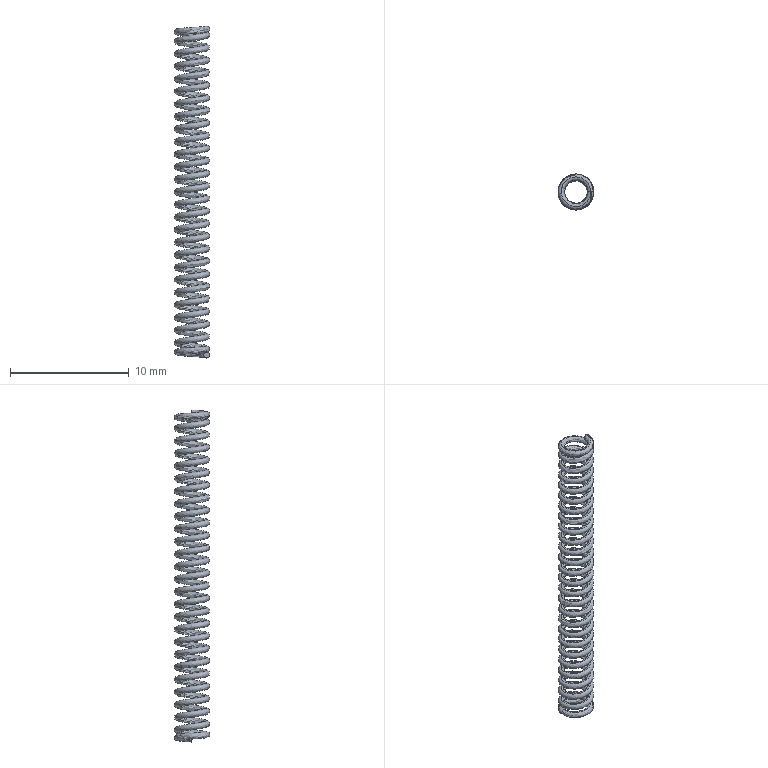Part | SolidWorks | features Helix 1, Sweep 1 | 1 solid | 4 faces | box 3 x 3 x 28.006 mm | volume 41.608 mm3 | spline 2 | plane 2